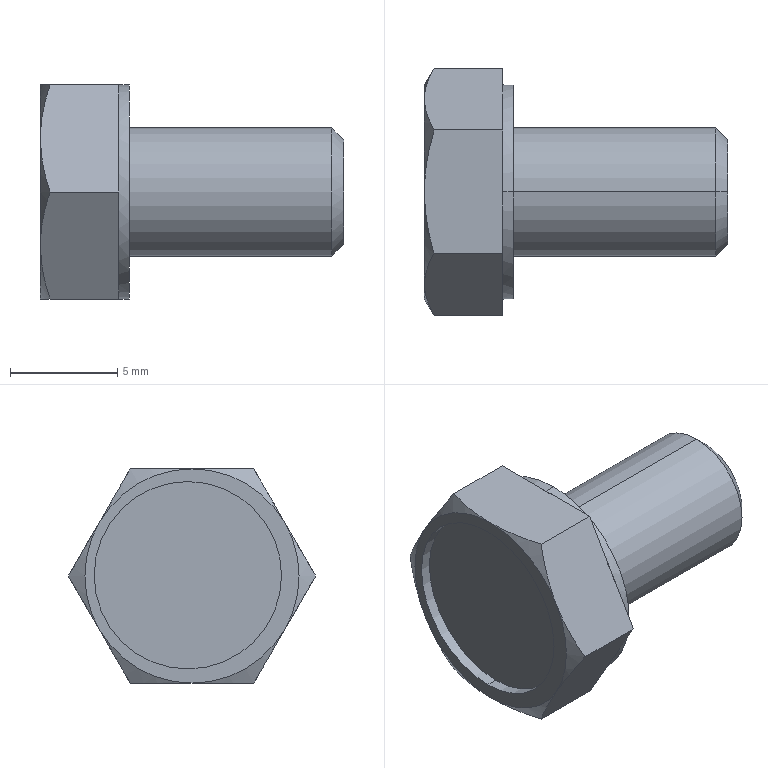Part | STEP file | formed hex screw_am_B18.2.3.2M - Formed hex screw, M6 x 1.0 x 10 --10WN | 1 solid | 30 faces | box 14.15 x 11.547 x 10 mm | volume 603.109 mm3 | plane 16 | cone 8 | cylinder 6 | commonest cylinder face diameters 6 x2 8.75 x2 10 x2